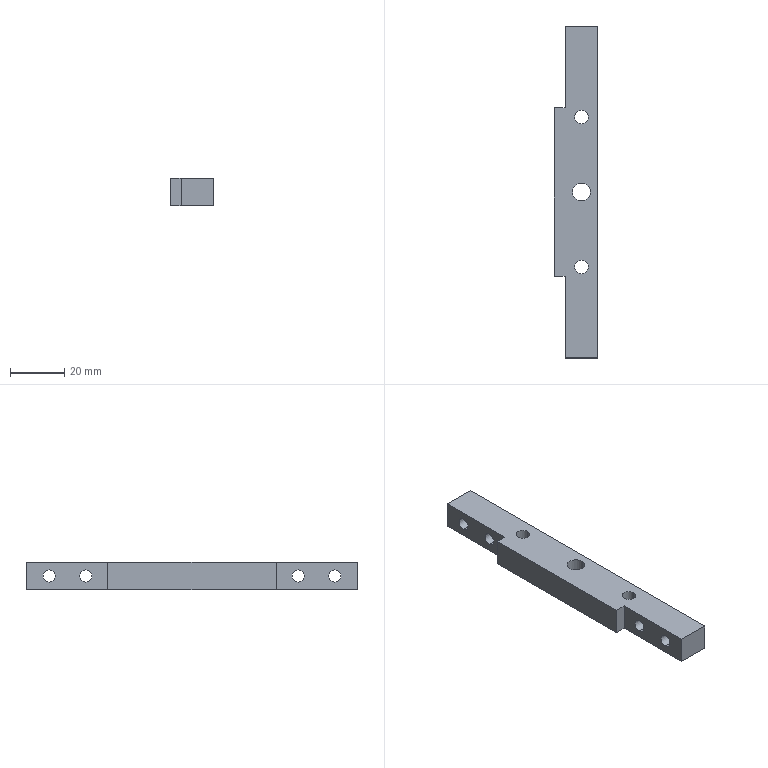Part | NX | features BREP 1 | 1 solid | 36 faces | box 16 x 122 x 10 mm | volume 15082 mm3 | cylinder 22 | plane 14 | commonest cylinder face diameters 4.5 x8 8 x8 5 x4 6.5 x2
STEP:
#1=CARTESIAN_POINT('',(-3.25,0.,0.));
#2=VERTEX_POINT('',#1);
#3=CARTESIAN_POINT('',(3.25,0.,0.));
#4=VERTEX_POINT('',#3);
#5=CARTESIAN_POINT('',(0.,0.,0.));
#6=DIRECTION('',(0.,0.,1.));
#7=DIRECTION('',(1.,0.,0.));
#8=AXIS2_PLACEMENT_3D('',#5,#6,#7);
#9=CIRCLE('',#8,3.25);
#10=EDGE_CURVE('',#2,#4,#9,.T.);
#11=ORIENTED_EDGE('',*,*,#10,.F.);
#12=CARTESIAN_POINT('',(-3.25,0.,10.));
#13=VERTEX_POINT('',#12);
#14=CARTESIAN_POINT('',(-3.25,0.,0.));
#15=DIRECTION('',(0.,0.,1.));
#16=VECTOR('',#15,1000.);
#17=LINE('',#14,#16);
#18=EDGE_CURVE('',#13,#2,#17,.F.);
#19=ORIENTED_EDGE('',*,*,#18,.F.);
#20=CARTESIAN_POINT('',(3.25,0.,10.));
#21=VERTEX_POINT('',#20);
#22=CARTESIAN_POINT('',(0.,0.,10.));
#23=DIRECTION('',(0.,0.,1.));
#24=DIRECTION('',(1.,0.,0.));
#25=AXIS2_PLACEMENT_3D('',#22,#23,#24);
#26=CIRCLE('',#25,3.25);
#27=EDGE_CURVE('',#13,#21,#26,.T.);
#28=ORIENTED_EDGE('',*,*,#27,.T.);
#29=CARTESIAN_POINT('',(3.25,0.,0.));
#30=DIRECTION('',(0.,0.,1.));
#31=VECTOR('',#30,1000.);
#32=LINE('',#29,#31);
#33=EDGE_CURVE('',#21,#4,#32,.F.);
#34=ORIENTED_EDGE('',*,*,#33,.T.);
#35=EDGE_LOOP('',(#11,#19,#28,#34));
#36=FACE_BOUND('',#35,.T.);
#37=CARTESIAN_POINT('',(0.,0.,0.));
#38=DIRECTION('',(0.,0.,1.));
#39=DIRECTION('',(1.,0.,0.));
#40=AXIS2_PLACEMENT_3D('',#37,#38,#39);
#41=CYLINDRICAL_SURFACE('',#40,3.25);
#42=ADVANCED_FACE('',(#36),#41,.F.);
#43=CARTESIAN_POINT('',(-2.5,27.5,0.));
#44=VERTEX_POINT('',#43);
#45=CARTESIAN_POINT('',(2.5,27.5,0.));
#46=VERTEX_POINT('',#45);
#47=CARTESIAN_POINT('',(0.,27.5,0.));
#48=DIRECTION('',(0.,0.,1.));
#49=DIRECTION('',(1.,0.,0.));
#50=AXIS2_PLACEMENT_3D('',#47,#48,#49);
#51=CIRCLE('',#50,2.5);
#52=EDGE_CURVE('',#44,#46,#51,.T.);
#53=ORIENTED_EDGE('',*,*,#52,.F.);
#54=CARTESIAN_POINT('',(-2.5,27.5,10.));
#55=VERTEX_POINT('',#54);
#56=CARTESIAN_POINT('',(-2.5,27.5,10.));
#57=DIRECTION('',(0.,0.,1.));
#58=VECTOR('',#57,1000.);
#59=LINE('',#56,#58);
#60=EDGE_CURVE('',#55,#44,#59,.F.);
#61=ORIENTED_EDGE('',*,*,#60,.F.);
#62=CARTESIAN_POINT('',(2.5,27.5,10.));
#63=VERTEX_POINT('',#62);
#64=CARTESIAN_POINT('',(0.,27.5,10.));
#65=DIRECTION('',(0.,0.,1.));
#66=DIRECTION('',(1.,0.,0.));
#67=AXIS2_PLACEMENT_3D('',#64,#65,#66);
#68=CIRCLE('',#67,2.5);
#69=EDGE_CURVE('',#55,#63,#68,.T.);
#70=ORIENTED_EDGE('',*,*,#69,.T.);
#71=CARTESIAN_POINT('',(2.5,27.5,10.));
#72=DIRECTION('',(0.,0.,1.));
#73=VECTOR('',#72,1000.);
#74=LINE('',#71,#73);
#75=EDGE_CURVE('',#63,#46,#74,.F.);
#76=ORIENTED_EDGE('',*,*,#75,.T.);
#77=EDGE_LOOP('',(#53,#61,#70,#76));
#78=FACE_BOUND('',#77,.T.);
#79=CARTESIAN_POINT('',(0.,27.5,10.));
#80=DIRECTION('',(0.,0.,1.));
#81=DIRECTION('',(1.,0.,0.));
#82=AXIS2_PLACEMENT_3D('',#79,#80,#81);
#83=CYLINDRICAL_SURFACE('',#82,2.5);
#84=ADVANCED_FACE('',(#78),#83,.F.);
#85=CARTESIAN_POINT('',(-2.5,-27.5,0.));
#86=VERTEX_POINT('',#85);
#87=CARTESIAN_POINT('',(2.5,-27.5,0.));
#88=VERTEX_POINT('',#87);
#89=CARTESIAN_POINT('',(0.,-27.5,0.));
#90=DIRECTION('',(0.,0.,1.));
#91=DIRECTION('',(1.,0.,0.));
#92=AXIS2_PLACEMENT_3D('',#89,#90,#91);
#93=CIRCLE('',#92,2.5);
#94=EDGE_CURVE('',#86,#88,#93,.T.);
#95=ORIENTED_EDGE('',*,*,#94,.F.);
#96=CARTESIAN_POINT('',(-2.5,-27.5,10.));
#97=VERTEX_POINT('',#96);
#98=CARTESIAN_POINT('',(-2.5,-27.5,10.));
#99=DIRECTION('',(0.,0.,1.));
#100=VECTOR('',#99,1000.);
#101=LINE('',#98,#100);
#102=EDGE_CURVE('',#97,#86,#101,.F.);
#103=ORIENTED_EDGE('',*,*,#102,.F.);
#104=CARTESIAN_POINT('',(2.5,-27.5,10.));
#105=VERTEX_POINT('',#104);
#106=CARTESIAN_POINT('',(0.,-27.5,10.));
#107=DIRECTION('',(0.,0.,1.));
#108=DIRECTION('',(1.,0.,0.));
#109=AXIS2_PLACEMENT_3D('',#106,#107,#108);
#110=CIRCLE('',#109,2.5);
#111=EDGE_CURVE('',#97,#105,#110,.T.);
#112=ORIENTED_EDGE('',*,*,#111,.T.);
#113=CARTESIAN_POINT('',(2.5,-27.5,10.));
#114=DIRECTION('',(0.,0.,1.));
#115=VECTOR('',#114,1000.);
#116=LINE('',#113,#115);
#117=EDGE_CURVE('',#105,#88,#116,.F.);
#118=ORIENTED_EDGE('',*,*,#117,.T.);
#119=EDGE_LOOP('',(#95,#103,#112,#118));
#120=FACE_BOUND('',#119,.T.);
#121=CARTESIAN_POINT('',(0.,-27.5,10.));
#122=DIRECTION('',(0.,0.,1.));
#123=DIRECTION('',(1.,0.,0.));
#124=AXIS2_PLACEMENT_3D('',#121,#122,#123);
#125=CYLINDRICAL_SURFACE('',#124,2.5);
#126=ADVANCED_FACE('',(#120),#125,.F.);
#127=CARTESIAN_POINT('',(2.,52.5,9.));
#128=VERTEX_POINT('',#127);
#129=CARTESIAN_POINT('',(2.,52.5,1.));
#130=VERTEX_POINT('',#129);
#131=CARTESIAN_POINT('',(2.,52.5,5.));
#132=DIRECTION('',(1.,0.,0.));
#133=DIRECTION('',(0.,0.,-1.));
#134=AXIS2_PLACEMENT_3D('',#131,#132,#133);
#135=CIRCLE('',#134,4.);
#136=EDGE_CURVE('',#128,#130,#135,.T.);
#137=ORIENTED_EDGE('',*,*,#136,.F.);
#138=CARTESIAN_POINT('',(6.,52.5,9.));
#139=VERTEX_POINT('',#138);
#140=CARTESIAN_POINT('',(6.,52.5,9.));
#141=DIRECTION('',(1.,0.,0.));
#142=VECTOR('',#141,1000.);
#143=LINE('',#140,#142);
#144=EDGE_CURVE('',#128,#139,#143,.T.);
#145=ORIENTED_EDGE('',*,*,#144,.T.);
#146=CARTESIAN_POINT('',(6.,52.5,1.));
#147=VERTEX_POINT('',#146);
#148=CARTESIAN_POINT('',(6.,52.5,5.));
#149=DIRECTION('',(1.,0.,0.));
#150=DIRECTION('',(0.,0.,-1.));
#151=AXIS2_PLACEMENT_3D('',#148,#149,#150);
#152=CIRCLE('',#151,4.);
#153=EDGE_CURVE('',#139,#147,#152,.T.);
#154=ORIENTED_EDGE('',*,*,#153,.T.);
#155=CARTESIAN_POINT('',(6.,52.5,1.));
#156=DIRECTION('',(1.,0.,0.));
#157=VECTOR('',#156,1000.);
#158=LINE('',#155,#157);
#159=EDGE_CURVE('',#130,#147,#158,.T.);
#160=ORIENTED_EDGE('',*,*,#159,.F.);
#161=EDGE_LOOP('',(#137,#145,#154,#160));
#162=FACE_BOUND('',#161,.T.);
#163=CARTESIAN_POINT('',(6.,52.5,5.));
#164=DIRECTION('',(1.,0.,0.));
#165=DIRECTION('',(0.,0.,-1.));
#166=AXIS2_PLACEMENT_3D('',#163,#164,#165);
#167=CYLINDRICAL_SURFACE('',#166,4.);
#168=ADVANCED_FACE('',(#162),#167,.F.);
#169=CARTESIAN_POINT('',(-6.,52.5,7.25));
#170=VERTEX_POINT('',#169);
#171=CARTESIAN_POINT('',(-6.,52.5,2.75));
#172=VERTEX_POINT('',#171);
#173=CARTESIAN_POINT('',(-6.,52.5,5.));
#174=DIRECTION('',(1.,0.,0.));
#175=DIRECTION('',(0.,1.,0.));
#176=AXIS2_PLACEMENT_3D('',#173,#174,#175);
#177=CIRCLE('',#176,2.25);
#178=EDGE_CURVE('',#170,#172,#177,.T.);
#179=ORIENTED_EDGE('',*,*,#178,.F.);
#180=CARTESIAN_POINT('',(2.,52.5,7.25));
#181=VERTEX_POINT('',#180);
#182=CARTESIAN_POINT('',(6.,52.5,7.25));
#183=DIRECTION('',(1.,0.,0.));
#184=VECTOR('',#183,1000.);
#185=LINE('',#182,#184);
#186=EDGE_CURVE('',#170,#181,#185,.T.);
#187=ORIENTED_EDGE('',*,*,#186,.T.);
#188=CARTESIAN_POINT('',(2.,52.5,2.75));
#189=VERTEX_POINT('',#188);
#190=CARTESIAN_POINT('',(2.,52.5,5.));
#191=DIRECTION('',(1.,0.,0.));
#192=DIRECTION('',(0.,0.,-1.));
#193=AXIS2_PLACEMENT_3D('',#190,#191,#192);
#194=CIRCLE('',#193,2.25);
#195=EDGE_CURVE('',#181,#189,#194,.T.);
#196=ORIENTED_EDGE('',*,*,#195,.T.);
#197=CARTESIAN_POINT('',(6.,52.5,2.75));
#198=DIRECTION('',(1.,0.,0.));
#199=VECTOR('',#198,1000.);
#200=LINE('',#197,#199);
#201=EDGE_CURVE('',#172,#189,#200,.T.);
#202=ORIENTED_EDGE('',*,*,#201,.F.);
#203=EDGE_LOOP('',(#179,#187,#196,#202));
#204=FACE_BOUND('',#203,.T.);
#205=CARTESIAN_POINT('',(6.,52.5,5.));
#206=DIRECTION('',(1.,0.,0.));
#207=DIRECTION('',(0.,0.,-1.));
#208=AXIS2_PLACEMENT_3D('',#205,#206,#207);
#209=CYLINDRICAL_SURFACE('',#208,2.25);
#210=ADVANCED_FACE('',(#204),#209,.F.);
#211=CARTESIAN_POINT('',(2.,39.,9.));
#212=VERTEX_POINT('',#211);
#213=CARTESIAN_POINT('',(2.,39.,1.));
#214=VERTEX_POINT('',#213);
#215=CARTESIAN_POINT('',(2.,39.,5.));
#216=DIRECTION('',(1.,0.,0.));
#217=DIRECTION('',(0.,0.,-1.));
#218=AXIS2_PLACEMENT_3D('',#215,#216,#217);
#219=CIRCLE('',#218,4.);
#220=EDGE_CURVE('',#212,#214,#219,.T.);
#221=ORIENTED_EDGE('',*,*,#220,.F.);
#222=CARTESIAN_POINT('',(6.,39.,9.));
#223=VERTEX_POINT('',#222);
#224=CARTESIAN_POINT('',(6.,39.,9.));
#225=DIRECTION('',(1.,0.,0.));
#226=VECTOR('',#225,1000.);
#227=LINE('',#224,#226);
#228=EDGE_CURVE('',#212,#223,#227,.T.);
#229=ORIENTED_EDGE('',*,*,#228,.T.);
#230=CARTESIAN_POINT('',(6.,39.,1.));
#231=VERTEX_POINT('',#230);
#232=CARTESIAN_POINT('',(6.,39.,5.));
#233=DIRECTION('',(1.,0.,0.));
#234=DIRECTION('',(0.,0.,-1.));
#235=AXIS2_PLACEMENT_3D('',#232,#233,#234);
#236=CIRCLE('',#235,4.);
#237=EDGE_CURVE('',#223,#231,#236,.T.);
#238=ORIENTED_EDGE('',*,*,#237,.T.);
#239=CARTESIAN_POINT('',(6.,39.,1.));
#240=DIRECTION('',(1.,0.,0.));
#241=VECTOR('',#240,1000.);
#242=LINE('',#239,#241);
#243=EDGE_CURVE('',#214,#231,#242,.T.);
#244=ORIENTED_EDGE('',*,*,#243,.F.);
#245=EDGE_LOOP('',(#221,#229,#238,#244));
#246=FACE_BOUND('',#245,.T.);
#247=CARTESIAN_POINT('',(6.,39.,5.));
#248=DIRECTION('',(1.,0.,0.));
#249=DIRECTION('',(0.,0.,-1.));
#250=AXIS2_PLACEMENT_3D('',#247,#248,#249);
#251=CYLINDRICAL_SURFACE('',#250,4.);
#252=ADVANCED_FACE('',(#246),#251,.F.);
#253=CARTESIAN_POINT('',(-6.,39.,7.25));
#254=VERTEX_POINT('',#253);
#255=CARTESIAN_POINT('',(-6.,39.,2.75));
#256=VERTEX_POINT('',#255);
#257=CARTESIAN_POINT('',(-6.,39.,5.));
#258=DIRECTION('',(1.,0.,0.));
#259=DIRECTION('',(0.,1.,0.));
#260=AXIS2_PLACEMENT_3D('',#257,#258,#259);
#261=CIRCLE('',#260,2.25);
#262=EDGE_CURVE('',#254,#256,#261,.T.);
#263=ORIENTED_EDGE('',*,*,#262,.F.);
#264=CARTESIAN_POINT('',(2.,39.,7.25));
#265=VERTEX_POINT('',#264);
#266=CARTESIAN_POINT('',(6.,39.,7.25));
#267=DIRECTION('',(1.,0.,0.));
#268=VECTOR('',#267,1000.);
#269=LINE('',#266,#268);
#270=EDGE_CURVE('',#254,#265,#269,.T.);
#271=ORIENTED_EDGE('',*,*,#270,.T.);
#272=CARTESIAN_POINT('',(2.,39.,2.75));
#273=VERTEX_POINT('',#272);
#274=CARTESIAN_POINT('',(2.,39.,5.));
#275=DIRECTION('',(1.,0.,0.));
#276=DIRECTION('',(0.,0.,-1.));
#277=AXIS2_PLACEMENT_3D('',#274,#275,#276);
#278=CIRCLE('',#277,2.25);
#279=EDGE_CURVE('',#265,#273,#278,.T.);
#280=ORIENTED_EDGE('',*,*,#279,.T.);
#281=CARTESIAN_POINT('',(6.,39.,2.75));
#282=DIRECTION('',(1.,0.,0.));
#283=VECTOR('',#282,1000.);
#284=LINE('',#281,#283);
#285=EDGE_CURVE('',#256,#273,#284,.T.);
#286=ORIENTED_EDGE('',*,*,#285,.F.);
#287=EDGE_LOOP('',(#263,#271,#280,#286));
#288=FACE_BOUND('',#287,.T.);
#289=CARTESIAN_POINT('',(6.,39.,5.));
#290=DIRECTION('',(1.,0.,0.));
#291=DIRECTION('',(0.,0.,-1.));
#292=AXIS2_PLACEMENT_3D('',#289,#290,#291);
#293=CYLINDRICAL_SURFACE('',#292,2.25);
#294=ADVANCED_FACE('',(#288),#293,.F.);
#295=CARTESIAN_POINT('',(2.,-39.,9.));
#296=VERTEX_POINT('',#295);
#297=CARTESIAN_POINT('',(2.,-39.,1.));
#298=VERTEX_POINT('',#297);
#299=CARTESIAN_POINT('',(2.,-39.,5.));
#300=DIRECTION('',(1.,0.,0.));
#301=DIRECTION('',(0.,0.,-1.));
#302=AXIS2_PLACEMENT_3D('',#299,#300,#301);
#303=CIRCLE('',#302,4.);
#304=EDGE_CURVE('',#296,#298,#303,.T.);
#305=ORIENTED_EDGE('',*,*,#304,.F.);
#306=CARTESIAN_POINT('',(6.,-39.,9.));
#307=VERTEX_POINT('',#306);
#308=CARTESIAN_POINT('',(6.,-39.,9.));
#309=DIRECTION('',(1.,0.,0.));
#310=VECTOR('',#309,1000.);
#311=LINE('',#308,#310);
#312=EDGE_CURVE('',#296,#307,#311,.T.);
#313=ORIENTED_EDGE('',*,*,#312,.T.);
#314=CARTESIAN_POINT('',(6.,-39.,1.));
#315=VERTEX_POINT('',#314);
#316=CARTESIAN_POINT('',(6.,-39.,5.));
#317=DIRECTION('',(1.,0.,0.));
#318=DIRECTION('',(0.,0.,-1.));
#319=AXIS2_PLACEMENT_3D('',#316,#317,#318);
#320=CIRCLE('',#319,4.);
#321=EDGE_CURVE('',#307,#315,#320,.T.);
#322=ORIENTED_EDGE('',*,*,#321,.T.);
#323=CARTESIAN_POINT('',(6.,-39.,1.));
#324=DIRECTION('',(1.,0.,0.));
#325=VECTOR('',#324,1000.);
#326=LINE('',#323,#325);
#327=EDGE_CURVE('',#298,#315,#326,.T.);
#328=ORIENTED_EDGE('',*,*,#327,.F.);
#329=EDGE_LOOP('',(#305,#313,#322,#328));
#330=FACE_BOUND('',#329,.T.);
#331=CARTESIAN_POINT('',(6.,-39.,5.));
#332=DIRECTION('',(1.,0.,0.));
#333=DIRECTION('',(0.,0.,-1.));
#334=AXIS2_PLACEMENT_3D('',#331,#332,#333);
#335=CYLINDRICAL_SURFACE('',#334,4.);
#336=ADVANCED_FACE('',(#330),#335,.F.);
#337=CARTESIAN_POINT('',(-6.,-39.,7.25));
#338=VERTEX_POINT('',#337);
#339=CARTESIAN_POINT('',(-6.,-39.,2.75));
#340=VERTEX_POINT('',#339);
#341=CARTESIAN_POINT('',(-6.,-39.,5.));
#342=DIRECTION('',(1.,0.,0.));
#343=DIRECTION('',(0.,1.,0.));
#344=AXIS2_PLACEMENT_3D('',#341,#342,#343);
#345=CIRCLE('',#344,2.25);
#346=EDGE_CURVE('',#338,#340,#345,.T.);
#347=ORIENTED_EDGE('',*,*,#346,.F.);
#348=CARTESIAN_POINT('',(2.,-39.,7.25));
#349=VERTEX_POINT('',#348);
#350=CARTESIAN_POINT('',(6.,-39.,7.25));
#351=DIRECTION('',(1.,0.,0.));
#352=VECTOR('',#351,1000.);
#353=LINE('',#350,#352);
#354=EDGE_CURVE('',#338,#349,#353,.T.);
#355=ORIENTED_EDGE('',*,*,#354,.T.);
#356=CARTESIAN_POINT('',(2.,-39.,2.75));
#357=VERTEX_POINT('',#356);
#358=CARTESIAN_POINT('',(2.,-39.,5.));
#359=DIRECTION('',(1.,0.,0.));
#360=DIRECTION('',(0.,0.,-1.));
#361=AXIS2_PLACEMENT_3D('',#358,#359,#360);
#362=CIRCLE('',#361,2.25);
#363=EDGE_CURVE('',#349,#357,#362,.T.);
#364=ORIENTED_EDGE('',*,*,#363,.T.);
#365=CARTESIAN_POINT('',(6.,-39.,2.75));
#366=DIRECTION('',(1.,0.,0.));
#367=VECTOR('',#366,1000.);
#368=LINE('',#365,#367);
#369=EDGE_CURVE('',#340,#357,#368,.T.);
#370=ORIENTED_EDGE('',*,*,#369,.F.);
#371=EDGE_LOOP('',(#347,#355,#364,#370));
#372=FACE_BOUND('',#371,.T.);
#373=CARTESIAN_POINT('',(6.,-39.,5.));
#374=DIRECTION('',(1.,0.,0.));
#375=DIRECTION('',(0.,0.,-1.));
#376=AXIS2_PLACEMENT_3D('',#373,#374,#375);
#377=CYLINDRICAL_SURFACE('',#376,2.25);
#378=ADVANCED_FACE('',(#372),#377,.F.);
#379=CARTESIAN_POINT('',(2.,-52.5,9.));
#380=VERTEX_POINT('',#379);
#381=CARTESIAN_POINT('',(2.,-52.5,1.));
#382=VERTEX_POINT('',#381);
#383=CARTESIAN_POINT('',(2.,-52.5,5.));
#384=DIRECTION('',(1.,0.,0.));
#385=DIRECTION('',(0.,0.,-1.));
#386=AXIS2_PLACEMENT_3D('',#383,#384,#385);
#387=CIRCLE('',#386,4.);
#388=EDGE_CURVE('',#380,#382,#387,.T.);
#389=ORIENTED_EDGE('',*,*,#388,.F.);
#390=CARTESIAN_POINT('',(6.,-52.5,9.));
#391=VERTEX_POINT('',#390);
#392=CARTESIAN_POINT('',(6.,-52.5,9.));
#393=DIRECTION('',(1.,0.,0.));
#394=VECTOR('',#393,1000.);
#395=LINE('',#392,#394);
#396=EDGE_CURVE('',#380,#391,#395,.T.);
#397=ORIENTED_EDGE('',*,*,#396,.T.);
#398=CARTESIAN_POINT('',(6.,-52.5,1.));
#399=VERTEX_POINT('',#398);
#400=CARTESIAN_POINT('',(6.,-52.5,5.));
#401=DIRECTION('',(1.,0.,0.));
#402=DIRECTION('',(0.,0.,-1.));
#403=AXIS2_PLACEMENT_3D('',#400,#401,#402);
#404=CIRCLE('',#403,4.);
#405=EDGE_CURVE('',#391,#399,#404,.T.);
#406=ORIENTED_EDGE('',*,*,#405,.T.);
#407=CARTESIAN_POINT('',(6.,-52.5,1.));
#408=DIRECTION('',(1.,0.,0.));
#409=VECTOR('',#408,1000.);
#410=LINE('',#407,#409);
#411=EDGE_CURVE('',#382,#399,#410,.T.);
#412=ORIENTED_EDGE('',*,*,#411,.F.);
#413=EDGE_LOOP('',(#389,#397,#406,#412));
#414=FACE_BOUND('',#413,.T.);
#415=CARTESIAN_POINT('',(6.,-52.5,5.));
#416=DIRECTION('',(1.,0.,0.));
#417=DIRECTION('',(0.,0.,-1.));
#418=AXIS2_PLACEMENT_3D('',#415,#416,#417);
#419=CYLINDRICAL_SURFACE('',#418,4.);
#420=ADVANCED_FACE('',(#414),#419,.F.);
#421=CARTESIAN_POINT('',(-6.,-52.5,7.25));
#422=VERTEX_POINT('',#421);
#423=CARTESIAN_POINT('',(-6.,-52.5,2.75));
#424=VERTEX_POINT('',#423);
#425=CARTESIAN_POINT('',(-6.,-52.5,5.));
#426=DIRECTION('',(1.,0.,0.));
#427=DIRECTION('',(0.,1.,0.));
#428=AXIS2_PLACEMENT_3D('',#425,#426,#427);
#429=CIRCLE('',#428,2.25);
#430=EDGE_CURVE('',#422,#424,#429,.T.);
#431=ORIENTED_EDGE('',*,*,#430,.F.);
#432=CARTESIAN_POINT('',(2.,-52.5,7.25));
#433=VERTEX_POINT('',#432);
#434=CARTESIAN_POINT('',(6.,-52.5,7.25));
#435=DIRECTION('',(1.,0.,0.));
#436=VECTOR('',#435,1000.);
#437=LINE('',#434,#436);
#438=EDGE_CURVE('',#422,#433,#437,.T.);
#439=ORIENTED_EDGE('',*,*,#438,.T.);
#440=CARTESIAN_POINT('',(2.,-52.5,2.75));
#441=VERTEX_POINT('',#440);
#442=CARTESIAN_POINT('',(2.,-52.5,5.));
#443=DIRECTION('',(1.,0.,0.));
#444=DIRECTION('',(0.,0.,-1.));
#445=AXIS2_PLACEMENT_3D('',#442,#443,#444);
#446=CIRCLE('',#445,2.25);
#447=EDGE_CURVE('',#433,#441,#446,.T.);
#448=ORIENTED_EDGE('',*,*,#447,.T.);
#449=CARTESIAN_POINT('',(6.,-52.5,2.75));
#450=DIRECTION('',(1.,0.,0.));
#451=VECTOR('',#450,1000.);
#452=LINE('',#449,#451);
#453=EDGE_CURVE('',#424,#441,#452,.T.);
#454=ORIENTED_EDGE('',*,*,#453,.F.);
#455=EDGE_LOOP('',(#431,#439,#448,#454));
#456=FACE_BOUND('',#455,.T.);
#457=CARTESIAN_POINT('',(6.,-52.5,5.));
#458=DIRECTION('',(1.,0.,0.));
#459=DIRECTION('',(0.,0.,-1.));
#460=AXIS2_PLACEMENT_3D('',#457,#458,#459);
#461=CYLINDRICAL_SURFACE('',#460,2.25);
#462=ADVANCED_FACE('',(#456),#461,.F.);
#463=CARTESIAN_POINT('',(6.,-61.,0.));
#464=VERTEX_POINT('',#463);
#465=CARTESIAN_POINT('',(6.,61.,0.));
#466=VERTEX_POINT('',#465);
#467=CARTESIAN_POINT('',(6.,61.,0.));
#468=DIRECTION('',(0.,1.,0.));
#469=VECTOR('',#468,1000.);
#470=LINE('',#467,#469);
#471=EDGE_CURVE('',#464,#466,#470,.T.);
#472=ORIENTED_EDGE('',*,*,#471,.T.);
#473=CARTESIAN_POINT('',(6.,61.,10.));
#474=VERTEX_POINT('',#473);
#475=CARTESIAN_POINT('',(6.,61.,10.));
#476=DIRECTION('',(0.,0.,-1.));
#477=VECTOR('',#476,1000.);
#478=LINE('',#475,#477);
#479=EDGE_CURVE('',#474,#466,#478,.T.);
#480=ORIENTED_EDGE('',*,*,#479,.F.);
#481=CARTESIAN_POINT('',(6.,-61.,10.));
#482=VERTEX_POINT('',#481);
#483=CARTESIAN_POINT('',(6.,61.,10.));
#484=DIRECTION('',(0.,1.,0.));
#485=VECTOR('',#484,1000.);
#486=LINE('',#483,#485);
#487=EDGE_CURVE('',#482,#474,#486,.T.);
#488=ORIENTED_EDGE('',*,*,#487,.F.);
#489=CARTESIAN_POINT('',(6.,-61.,10.));
#490=DIRECTION('',(0.,0.,-1.));
#491=VECTOR('',#490,1000.);
#492=LINE('',#489,#491);
#493=EDGE_CURVE('',#482,#464,#492,.T.);
#494=ORIENTED_EDGE('',*,*,#493,.T.);
#495=EDGE_LOOP('',(#472,#480,#488,#494));
#496=FACE_BOUND('',#495,.T.);
#497=CARTESIAN_POINT('',(6.,52.5,5.));
#498=DIRECTION('',(1.,0.,0.));
#499=DIRECTION('',(0.,0.,-1.));
#500=AXIS2_PLACEMENT_3D('',#497,#498,#499);
#501=CIRCLE('',#500,4.);
#502=EDGE_CURVE('',#147,#139,#501,.T.);
#503=ORIENTED_EDGE('',*,*,#502,.F.);
#504=ORIENTED_EDGE('',*,*,#153,.F.);
#505=EDGE_LOOP('',(#503,#504));
#506=FACE_BOUND('',#505,.T.);
#507=CARTESIAN_POINT('',(6.,39.,5.));
#508=DIRECTION('',(1.,0.,0.));
#509=DIRECTION('',(0.,0.,-1.));
#510=AXIS2_PLACEMENT_3D('',#507,#508,#509);
#511=CIRCLE('',#510,4.);
#512=EDGE_CURVE('',#231,#223,#511,.T.);
#513=ORIENTED_EDGE('',*,*,#512,.F.);
#514=ORIENTED_EDGE('',*,*,#237,.F.);
#515=EDGE_LOOP('',(#513,#514));
#516=FACE_BOUND('',#515,.T.);
#517=CARTESIAN_POINT('',(6.,-39.,5.));
#518=DIRECTION('',(1.,0.,0.));
#519=DIRECTION('',(0.,0.,-1.));
#520=AXIS2_PLACEMENT_3D('',#517,#518,#519);
#521=CIRCLE('',#520,4.);
#522=EDGE_CURVE('',#315,#307,#521,.T.);
#523=ORIENTED_EDGE('',*,*,#522,.F.);
#524=ORIENTED_EDGE('',*,*,#321,.F.);
#525=EDGE_LOOP('',(#523,#524));
#526=FACE_BOUND('',#525,.T.);
#527=CARTESIAN_POINT('',(6.,-52.5,5.));
#528=DIRECTION('',(1.,0.,0.));
#529=DIRECTION('',(0.,0.,-1.));
#530=AXIS2_PLACEMENT_3D('',#527,#528,#529);
#531=CIRCLE('',#530,4.);
#532=EDGE_CURVE('',#399,#391,#531,.T.);
#533=ORIENTED_EDGE('',*,*,#532,.F.);
#534=ORIENTED_EDGE('',*,*,#405,.F.);
#535=EDGE_LOOP('',(#533,#534));
#536=FACE_BOUND('',#535,.T.);
#537=CARTESIAN_POINT('',(6.,61.,10.));
#538=DIRECTION('',(-1.,0.,0.));
#539=DIRECTION('',(0.,0.,1.));
#540=AXIS2_PLACEMENT_3D('',#537,#538,#539);
#541=PLANE('',#540);
#542=ADVANCED_FACE('',(#496,#506,#516,#526,#536),#541,.F.);
#543=CARTESIAN_POINT('',(-6.,61.,0.));
#544=VERTEX_POINT('',#543);
#545=CARTESIAN_POINT('',(6.,61.,0.));
#546=DIRECTION('',(-1.,0.,0.));
#547=VECTOR('',#546,1000.);
#548=LINE('',#545,#547);
#549=EDGE_CURVE('',#466,#544,#548,.T.);
#550=ORIENTED_EDGE('',*,*,#549,.T.);
#551=CARTESIAN_POINT('',(-6.,61.,10.));
#552=VERTEX_POINT('',#551);
#553=CARTESIAN_POINT('',(-6.,61.,10.));
#554=DIRECTION('',(0.,0.,-1.));
#555=VECTOR('',#554,1000.);
#556=LINE('',#553,#555);
#557=EDGE_CURVE('',#552,#544,#556,.T.);
#558=ORIENTED_EDGE('',*,*,#557,.F.);
#559=CARTESIAN_POINT('',(6.,61.,10.));
#560=DIRECTION('',(-1.,0.,0.));
#561=VECTOR('',#560,1000.);
#562=LINE('',#559,#561);
#563=EDGE_CURVE('',#474,#552,#562,.T.);
#564=ORIENTED_EDGE('',*,*,#563,.F.);
#565=ORIENTED_EDGE('',*,*,#479,.T.);
#566=EDGE_LOOP('',(#550,#558,#564,#565));
#567=FACE_BOUND('',#566,.T.);
#568=CARTESIAN_POINT('',(6.,61.,10.));
#569=DIRECTION('',(0.,-1.,0.));
#570=DIRECTION('',(0.,0.,-1.));
#571=AXIS2_PLACEMENT_3D('',#568,#569,#570);
#572=PLANE('',#571);
#573=ADVANCED_FACE('',(#567),#572,.F.);
#574=CARTESIAN_POINT('',(-6.,31.,0.));
#575=VERTEX_POINT('',#574);
#576=CARTESIAN_POINT('',(-6.,61.,0.));
#577=DIRECTION('',(0.,-1.,0.));
#578=VECTOR('',#577,1000.);
#579=LINE('',#576,#578);
#580=EDGE_CURVE('',#544,#575,#579,.T.);
#581=ORIENTED_EDGE('',*,*,#580,.T.);
#582=CARTESIAN_POINT('',(-6.,31.,10.));
#583=VERTEX_POINT('',#582);
#584=CARTESIAN_POINT('',(-6.,31.,10.));
#585=DIRECTION('',(0.,0.,-1.));
#586=VECTOR('',#585,1000.);
#587=LINE('',#584,#586);
#588=EDGE_CURVE('',#583,#575,#587,.T.);
#589=ORIENTED_EDGE('',*,*,#588,.F.);
#590=CARTESIAN_POINT('',(-6.,61.,10.));
#591=DIRECTION('',(0.,-1.,0.));
#592=VECTOR('',#591,1000.);
#593=LINE('',#590,#592);
#594=EDGE_CURVE('',#552,#583,#593,.T.);
#595=ORIENTED_EDGE('',*,*,#594,.F.);
#596=ORIENTED_EDGE('',*,*,#557,.T.);
#597=EDGE_LOOP('',(#581,#589,#595,#596));
#598=FACE_BOUND('',#597,.T.);
#599=CARTESIAN_POINT('',(-6.,52.5,5.));
#600=DIRECTION('',(1.,0.,0.));
#601=DIRECTION('',(0.,1.,0.));
#602=AXIS2_PLACEMENT_3D('',#599,#600,#601);
#603=CIRCLE('',#602,2.25);
#604=EDGE_CURVE('',#172,#170,#603,.T.);
#605=ORIENTED_EDGE('',*,*,#604,.T.);
#606=ORIENTED_EDGE('',*,*,#178,.T.);
#607=EDGE_LOOP('',(#605,#606));
#608=FACE_BOUND('',#607,.T.);
#609=CARTESIAN_POINT('',(-6.,39.,5.));
#610=DIRECTION('',(1.,0.,0.));
#611=DIRECTION('',(0.,1.,0.));
#612=AXIS2_PLACEMENT_3D('',#609,#610,#611);
#613=CIRCLE('',#612,2.25);
#614=EDGE_CURVE('',#256,#254,#613,.T.);
#615=ORIENTED_EDGE('',*,*,#614,.T.);
#616=ORIENTED_EDGE('',*,*,#262,.T.);
#617=EDGE_LOOP('',(#615,#616));
#618=FACE_BOUND('',#617,.T.);
#619=CARTESIAN_POINT('',(-6.,61.,10.));
#620=DIRECTION('',(1.,0.,0.));
#621=DIRECTION('',(0.,1.,0.));
#622=AXIS2_PLACEMENT_3D('',#619,#620,#621);
#623=PLANE('',#622);
#624=ADVANCED_FACE('',(#598,#608,#618),#623,.F.);
#625=CARTESIAN_POINT('',(-10.,31.,0.));
#626=VERTEX_POINT('',#625);
#627=CARTESIAN_POINT('',(-6.,31.,0.));
#628=DIRECTION('',(-1.,0.,0.));
#629=VECTOR('',#628,1000.);
#630=LINE('',#627,#629);
#631=EDGE_CURVE('',#575,#626,#630,.T.);
#632=ORIENTED_EDGE('',*,*,#631,.T.);
#633=CARTESIAN_POINT('',(-10.,31.,10.));
#634=VERTEX_POINT('',#633);
#635=CARTESIAN_POINT('',(-10.,31.,10.));
#636=DIRECTION('',(0.,0.,-1.));
#637=VECTOR('',#636,1000.);
#638=LINE('',#635,#637);
#639=EDGE_CURVE('',#634,#626,#638,.T.);
#640=ORIENTED_EDGE('',*,*,#639,.F.);
#641=CARTESIAN_POINT('',(-6.,31.,10.));
#642=DIRECTION('',(-1.,0.,0.));
#643=VECTOR('',#642,1000.);
#644=LINE('',#641,#643);
#645=EDGE_CURVE('',#583,#634,#644,.T.);
#646=ORIENTED_EDGE('',*,*,#645,.F.);
#647=ORIENTED_EDGE('',*,*,#588,.T.);
#648=EDGE_LOOP('',(#632,#640,#646,#647));
#649=FACE_BOUND('',#648,.T.);
#650=CARTESIAN_POINT('',(-6.,31.,10.));
#651=DIRECTION('',(0.,-1.,0.));
#652=DIRECTION('',(0.,0.,-1.));
#653=AXIS2_PLACEMENT_3D('',#650,#651,#652);
#654=PLANE('',#653);
#655=ADVANCED_FACE('',(#649),#654,.F.);
#656=CARTESIAN_POINT('',(-10.,-31.,0.));
#657=VERTEX_POINT('',#656);
#658=CARTESIAN_POINT('',(-10.,31.,0.));
#659=DIRECTION('',(0.,-1.,0.));
#660=VECTOR('',#659,1000.);
#661=LINE('',#658,#660);
#662=EDGE_CURVE('',#626,#657,#661,.T.);
#663=ORIENTED_EDGE('',*,*,#662,.T.);
#664=CARTESIAN_POINT('',(-10.,-31.,10.));
#665=VERTEX_POINT('',#664);
#666=CARTESIAN_POINT('',(-10.,-31.,10.));
#667=DIRECTION('',(0.,0.,-1.));
#668=VECTOR('',#667,1000.);
#669=LINE('',#666,#668);
#670=EDGE_CURVE('',#665,#657,#669,.T.);
#671=ORIENTED_EDGE('',*,*,#670,.F.);
#672=CARTESIAN_POINT('',(-10.,31.,10.));
#673=DIRECTION('',(0.,-1.,0.));
#674=VECTOR('',#673,1000.);
#675=LINE('',#672,#674);
#676=EDGE_CURVE('',#634,#665,#675,.T.);
#677=ORIENTED_EDGE('',*,*,#676,.F.);
#678=ORIENTED_EDGE('',*,*,#639,.T.);
#679=EDGE_LOOP('',(#663,#671,#677,#678));
#680=FACE_BOUND('',#679,.T.);
#681=CARTESIAN_POINT('',(-10.,31.,10.));
#682=DIRECTION('',(1.,0.,0.));
#683=DIRECTION('',(0.,1.,0.));
#684=AXIS2_PLACEMENT_3D('',#681,#682,#683);
#685=PLANE('',#684);
#686=ADVANCED_FACE('',(#680),#685,.F.);
#687=CARTESIAN_POINT('',(-6.,-31.,0.));
#688=VERTEX_POINT('',#687);
#689=CARTESIAN_POINT('',(-6.,-31.,0.));
#690=DIRECTION('',(1.,0.,0.));
#691=VECTOR('',#690,1000.);
#692=LINE('',#689,#691);
#693=EDGE_CURVE('',#657,#688,#692,.T.);
#694=ORIENTED_EDGE('',*,*,#693,.T.);
#695=CARTESIAN_POINT('',(-6.,-31.,10.));
#696=VERTEX_POINT('',#695);
#697=CARTESIAN_POINT('',(-6.,-31.,10.));
#698=DIRECTION('',(0.,0.,-1.));
#699=VECTOR('',#698,1000.);
#700=LINE('',#697,#699);
#701=EDGE_CURVE('',#696,#688,#700,.T.);
#702=ORIENTED_EDGE('',*,*,#701,.F.);
#703=CARTESIAN_POINT('',(-6.,-31.,10.));
#704=DIRECTION('',(1.,0.,0.));
#705=VECTOR('',#704,1000.);
#706=LINE('',#703,#705);
#707=EDGE_CURVE('',#665,#696,#706,.T.);
#708=ORIENTED_EDGE('',*,*,#707,.F.);
#709=ORIENTED_EDGE('',*,*,#670,.T.);
#710=EDGE_LOOP('',(#694,#702,#708,#709));
#711=FACE_BOUND('',#710,.T.);
#712=CARTESIAN_POINT('',(-6.,-31.,10.));
#713=DIRECTION('',(0.,1.,0.));
#714=DIRECTION('',(1.,0.,0.));
#715=AXIS2_PLACEMENT_3D('',#712,#713,#714);
#716=PLANE('',#715);
#717=ADVANCED_FACE('',(#711),#716,.F.);
#718=CARTESIAN_POINT('',(-6.,-61.,0.));
#719=VERTEX_POINT('',#718);
#720=CARTESIAN_POINT('',(-6.,-31.,0.));
#721=DIRECTION('',(0.,-1.,0.));
#722=VECTOR('',#721,1000.);
#723=LINE('',#720,#722);
#724=EDGE_CURVE('',#688,#719,#723,.T.);
#725=ORIENTED_EDGE('',*,*,#724,.T.);
#726=CARTESIAN_POINT('',(-6.,-61.,10.));
#727=VERTEX_POINT('',#726);
#728=CARTESIAN_POINT('',(-6.,-61.,10.));
#729=DIRECTION('',(0.,0.,-1.));
#730=VECTOR('',#729,1000.);
#731=LINE('',#728,#730);
#732=EDGE_CURVE('',#727,#719,#731,.T.);
#733=ORIENTED_EDGE('',*,*,#732,.F.);
#734=CARTESIAN_POINT('',(-6.,-31.,10.));
#735=DIRECTION('',(0.,-1.,0.));
#736=VECTOR('',#735,1000.);
#737=LINE('',#734,#736);
#738=EDGE_CURVE('',#696,#727,#737,.T.);
#739=ORIENTED_EDGE('',*,*,#738,.F.);
#740=ORIENTED_EDGE('',*,*,#701,.T.);
#741=EDGE_LOOP('',(#725,#733,#739,#740));
#742=FACE_BOUND('',#741,.T.);
#743=CARTESIAN_POINT('',(-6.,-39.,5.));
#744=DIRECTION('',(1.,0.,0.));
#745=DIRECTION('',(0.,1.,0.));
#746=AXIS2_PLACEMENT_3D('',#743,#744,#745);
#747=CIRCLE('',#746,2.25);
#748=EDGE_CURVE('',#340,#338,#747,.T.);
#749=ORIENTED_EDGE('',*,*,#748,.T.);
#750=ORIENTED_EDGE('',*,*,#346,.T.);
#751=EDGE_LOOP('',(#749,#750));
#752=FACE_BOUND('',#751,.T.);
#753=CARTESIAN_POINT('',(-6.,-52.5,5.));
#754=DIRECTION('',(1.,0.,0.));
#755=DIRECTION('',(0.,1.,0.));
#756=AXIS2_PLACEMENT_3D('',#753,#754,#755);
#757=CIRCLE('',#756,2.25);
#758=EDGE_CURVE('',#424,#422,#757,.T.);
#759=ORIENTED_EDGE('',*,*,#758,.T.);
#760=ORIENTED_EDGE('',*,*,#430,.T.);
#761=EDGE_LOOP('',(#759,#760));
#762=FACE_BOUND('',#761,.T.);
#763=CARTESIAN_POINT('',(-6.,-31.,10.));
#764=DIRECTION('',(1.,0.,0.));
#765=DIRECTION('',(0.,-1.,0.));
#766=AXIS2_PLACEMENT_3D('',#763,#764,#765);
#767=PLANE('',#766);
#768=ADVANCED_FACE('',(#742,#752,#762),#767,.F.);
#769=CARTESIAN_POINT('',(6.,-61.,0.));
#770=DIRECTION('',(1.,0.,0.));
#771=VECTOR('',#770,1000.);
#772=LINE('',#769,#771);
#773=EDGE_CURVE('',#719,#464,#772,.T.);
#774=ORIENTED_EDGE('',*,*,#773,.T.);
#775=ORIENTED_EDGE('',*,*,#493,.F.);
#776=CARTESIAN_POINT('',(6.,-61.,10.));
#777=DIRECTION('',(1.,0.,0.));
#778=VECTOR('',#777,1000.);
#779=LINE('',#776,#778);
#780=EDGE_CURVE('',#727,#482,#779,.T.);
#781=ORIENTED_EDGE('',*,*,#780,.F.);
#782=ORIENTED_EDGE('',*,*,#732,.T.);
#783=EDGE_LOOP('',(#774,#775,#781,#782));
#784=FACE_BOUND('',#783,.T.);
#785=CARTESIAN_POINT('',(6.,-61.,10.));
#786=DIRECTION('',(0.,1.,0.));
#787=DIRECTION('',(1.,0.,0.));
#788=AXIS2_PLACEMENT_3D('',#785,#786,#787);
#789=PLANE('',#788);
#790=ADVANCED_FACE('',(#784),#789,.F.);
#791=ORIENTED_EDGE('',*,*,#487,.T.);
#792=ORIENTED_EDGE('',*,*,#563,.T.);
#793=ORIENTED_EDGE('',*,*,#594,.T.);
#794=ORIENTED_EDGE('',*,*,#645,.T.);
#795=ORIENTED_EDGE('',*,*,#676,.T.);
#796=ORIENTED_EDGE('',*,*,#707,.T.);
#797=ORIENTED_EDGE('',*,*,#738,.T.);
#798=ORIENTED_EDGE('',*,*,#780,.T.);
#799=EDGE_LOOP('',(#791,#792,#793,#794,#795,#796,#797,#798));
#800=FACE_BOUND('',#799,.T.);
#801=CARTESIAN_POINT('',(0.,0.,10.));
#802=DIRECTION('',(0.,0.,1.));
#803=DIRECTION('',(1.,0.,0.));
#804=AXIS2_PLACEMENT_3D('',#801,#802,#803);
#805=CIRCLE('',#804,3.25);
#806=EDGE_CURVE('',#21,#13,#805,.T.);
#807=ORIENTED_EDGE('',*,*,#806,.F.);
#808=ORIENTED_EDGE('',*,*,#27,.F.);
#809=EDGE_LOOP('',(#807,#808));
#810=FACE_BOUND('',#809,.T.);
#811=CARTESIAN_POINT('',(0.,27.5,10.));
#812=DIRECTION('',(0.,0.,1.));
#813=DIRECTION('',(1.,0.,0.));
#814=AXIS2_PLACEMENT_3D('',#811,#812,#813);
#815=CIRCLE('',#814,2.5);
#816=EDGE_CURVE('',#63,#55,#815,.T.);
#817=ORIENTED_EDGE('',*,*,#816,.F.);
#818=ORIENTED_EDGE('',*,*,#69,.F.);
#819=EDGE_LOOP('',(#817,#818));
#820=FACE_BOUND('',#819,.T.);
#821=CARTESIAN_POINT('',(0.,-27.5,10.));
#822=DIRECTION('',(0.,0.,1.));
#823=DIRECTION('',(1.,0.,0.));
#824=AXIS2_PLACEMENT_3D('',#821,#822,#823);
#825=CIRCLE('',#824,2.5);
#826=EDGE_CURVE('',#105,#97,#825,.T.);
#827=ORIENTED_EDGE('',*,*,#826,.F.);
#828=ORIENTED_EDGE('',*,*,#111,.F.);
#829=EDGE_LOOP('',(#827,#828));
#830=FACE_BOUND('',#829,.T.);
#831=CARTESIAN_POINT('',(6.,-61.,10.));
#832=DIRECTION('',(0.,0.,-1.));
#833=DIRECTION('',(0.,-1.,0.));
#834=AXIS2_PLACEMENT_3D('',#831,#832,#833);
#835=PLANE('',#834);
#836=ADVANCED_FACE('',(#800,#810,#820,#830),#835,.F.);
#837=ORIENTED_EDGE('',*,*,#471,.F.);
#838=ORIENTED_EDGE('',*,*,#773,.F.);
#839=ORIENTED_EDGE('',*,*,#724,.F.);
#840=ORIENTED_EDGE('',*,*,#693,.F.);
#841=ORIENTED_EDGE('',*,*,#662,.F.);
#842=ORIENTED_EDGE('',*,*,#631,.F.);
#843=ORIENTED_EDGE('',*,*,#580,.F.);
#844=ORIENTED_EDGE('',*,*,#549,.F.);
#845=EDGE_LOOP('',(#837,#838,#839,#840,#841,#842,#843,#844));
#846=FACE_BOUND('',#845,.T.);
#847=CARTESIAN_POINT('',(0.,0.,0.));
#848=DIRECTION('',(0.,0.,1.));
#849=DIRECTION('',(1.,0.,0.));
#850=AXIS2_PLACEMENT_3D('',#847,#848,#849);
#851=CIRCLE('',#850,3.25);
#852=EDGE_CURVE('',#4,#2,#851,.T.);
#853=ORIENTED_EDGE('',*,*,#852,.T.);
#854=ORIENTED_EDGE('',*,*,#10,.T.);
#855=EDGE_LOOP('',(#853,#854));
#856=FACE_BOUND('',#855,.T.);
#857=CARTESIAN_POINT('',(0.,27.5,0.));
#858=DIRECTION('',(0.,0.,1.));
#859=DIRECTION('',(1.,0.,0.));
#860=AXIS2_PLACEMENT_3D('',#857,#858,#859);
#861=CIRCLE('',#860,2.5);
#862=EDGE_CURVE('',#46,#44,#861,.T.);
#863=ORIENTED_EDGE('',*,*,#862,.T.);
#864=ORIENTED_EDGE('',*,*,#52,.T.);
#865=EDGE_LOOP('',(#863,#864));
#866=FACE_BOUND('',#865,.T.);
#867=CARTESIAN_POINT('',(0.,-27.5,0.));
#868=DIRECTION('',(0.,0.,1.));
#869=DIRECTION('',(1.,0.,0.));
#870=AXIS2_PLACEMENT_3D('',#867,#868,#869);
#871=CIRCLE('',#870,2.5);
#872=EDGE_CURVE('',#88,#86,#871,.T.);
#873=ORIENTED_EDGE('',*,*,#872,.T.);
#874=ORIENTED_EDGE('',*,*,#94,.T.);
#875=EDGE_LOOP('',(#873,#874));
#876=FACE_BOUND('',#875,.T.);
#877=CARTESIAN_POINT('',(6.,-61.,0.));
#878=DIRECTION('',(0.,0.,-1.));
#879=DIRECTION('',(0.,-1.,0.));
#880=AXIS2_PLACEMENT_3D('',#877,#878,#879);
#881=PLANE('',#880);
#882=ADVANCED_FACE('',(#846,#856,#866,#876),#881,.T.);
#883=ORIENTED_EDGE('',*,*,#438,.F.);
#884=ORIENTED_EDGE('',*,*,#758,.F.);
#885=ORIENTED_EDGE('',*,*,#453,.T.);
#886=CARTESIAN_POINT('',(2.,-52.5,5.));
#887=DIRECTION('',(1.,0.,0.));
#888=DIRECTION('',(0.,0.,-1.));
#889=AXIS2_PLACEMENT_3D('',#886,#887,#888);
#890=CIRCLE('',#889,2.25);
#891=EDGE_CURVE('',#441,#433,#890,.T.);
#892=ORIENTED_EDGE('',*,*,#891,.T.);
#893=EDGE_LOOP('',(#883,#884,#885,#892));
#894=FACE_BOUND('',#893,.T.);
#895=CARTESIAN_POINT('',(6.,-52.5,5.));
#896=DIRECTION('',(1.,0.,0.));
#897=DIRECTION('',(0.,0.,-1.));
#898=AXIS2_PLACEMENT_3D('',#895,#896,#897);
#899=CYLINDRICAL_SURFACE('',#898,2.25);
#900=ADVANCED_FACE('',(#894),#899,.F.);
#901=CARTESIAN_POINT('',(2.,-52.5,5.));
#902=DIRECTION('',(1.,0.,0.));
#903=DIRECTION('',(0.,0.,-1.));
#904=AXIS2_PLACEMENT_3D('',#901,#902,#903);
#905=CIRCLE('',#904,4.);
#906=EDGE_CURVE('',#382,#380,#905,.T.);
#907=ORIENTED_EDGE('',*,*,#906,.T.);
#908=ORIENTED_EDGE('',*,*,#388,.T.);
#909=EDGE_LOOP('',(#907,#908));
#910=FACE_BOUND('',#909,.T.);
#911=ORIENTED_EDGE('',*,*,#891,.F.);
#912=ORIENTED_EDGE('',*,*,#447,.F.);
#913=EDGE_LOOP('',(#911,#912));
#914=FACE_BOUND('',#913,.T.);
#915=CARTESIAN_POINT('',(2.,-50.25,5.));
#916=DIRECTION('',(-1.,0.,0.));
#917=DIRECTION('',(0.,0.,1.));
#918=AXIS2_PLACEMENT_3D('',#915,#916,#917);
#919=PLANE('',#918);
#920=ADVANCED_FACE('',(#910,#914),#919,.F.);
#921=ORIENTED_EDGE('',*,*,#396,.F.);
#922=ORIENTED_EDGE('',*,*,#906,.F.);
#923=ORIENTED_EDGE('',*,*,#411,.T.);
#924=ORIENTED_EDGE('',*,*,#532,.T.);
#925=EDGE_LOOP('',(#921,#922,#923,#924));
#926=FACE_BOUND('',#925,.T.);
#927=CARTESIAN_POINT('',(6.,-52.5,5.));
#928=DIRECTION('',(1.,0.,0.));
#929=DIRECTION('',(0.,0.,-1.));
#930=AXIS2_PLACEMENT_3D('',#927,#928,#929);
#931=CYLINDRICAL_SURFACE('',#930,4.);
#932=ADVANCED_FACE('',(#926),#931,.F.);
#933=ORIENTED_EDGE('',*,*,#354,.F.);
#934=ORIENTED_EDGE('',*,*,#748,.F.);
#935=ORIENTED_EDGE('',*,*,#369,.T.);
#936=CARTESIAN_POINT('',(2.,-39.,5.));
#937=DIRECTION('',(1.,0.,0.));
#938=DIRECTION('',(0.,0.,-1.));
#939=AXIS2_PLACEMENT_3D('',#936,#937,#938);
#940=CIRCLE('',#939,2.25);
#941=EDGE_CURVE('',#357,#349,#940,.T.);
#942=ORIENTED_EDGE('',*,*,#941,.T.);
#943=EDGE_LOOP('',(#933,#934,#935,#942));
#944=FACE_BOUND('',#943,.T.);
#945=CARTESIAN_POINT('',(6.,-39.,5.));
#946=DIRECTION('',(1.,0.,0.));
#947=DIRECTION('',(0.,0.,-1.));
#948=AXIS2_PLACEMENT_3D('',#945,#946,#947);
#949=CYLINDRICAL_SURFACE('',#948,2.25);
#950=ADVANCED_FACE('',(#944),#949,.F.);
#951=CARTESIAN_POINT('',(2.,-39.,5.));
#952=DIRECTION('',(1.,0.,0.));
#953=DIRECTION('',(0.,0.,-1.));
#954=AXIS2_PLACEMENT_3D('',#951,#952,#953);
#955=CIRCLE('',#954,4.);
#956=EDGE_CURVE('',#298,#296,#955,.T.);
#957=ORIENTED_EDGE('',*,*,#956,.T.);
#958=ORIENTED_EDGE('',*,*,#304,.T.);
#959=EDGE_LOOP('',(#957,#958));
#960=FACE_BOUND('',#959,.T.);
#961=ORIENTED_EDGE('',*,*,#941,.F.);
#962=ORIENTED_EDGE('',*,*,#363,.F.);
#963=EDGE_LOOP('',(#961,#962));
#964=FACE_BOUND('',#963,.T.);
#965=CARTESIAN_POINT('',(2.,-36.75,5.));
#966=DIRECTION('',(-1.,0.,0.));
#967=DIRECTION('',(0.,0.,1.));
#968=AXIS2_PLACEMENT_3D('',#965,#966,#967);
#969=PLANE('',#968);
#970=ADVANCED_FACE('',(#960,#964),#969,.F.);
#971=ORIENTED_EDGE('',*,*,#312,.F.);
#972=ORIENTED_EDGE('',*,*,#956,.F.);
#973=ORIENTED_EDGE('',*,*,#327,.T.);
#974=ORIENTED_EDGE('',*,*,#522,.T.);
#975=EDGE_LOOP('',(#971,#972,#973,#974));
#976=FACE_BOUND('',#975,.T.);
#977=CARTESIAN_POINT('',(6.,-39.,5.));
#978=DIRECTION('',(1.,0.,0.));
#979=DIRECTION('',(0.,0.,-1.));
#980=AXIS2_PLACEMENT_3D('',#977,#978,#979);
#981=CYLINDRICAL_SURFACE('',#980,4.);
#982=ADVANCED_FACE('',(#976),#981,.F.);
#983=ORIENTED_EDGE('',*,*,#270,.F.);
#984=ORIENTED_EDGE('',*,*,#614,.F.);
#985=ORIENTED_EDGE('',*,*,#285,.T.);
#986=CARTESIAN_POINT('',(2.,39.,5.));
#987=DIRECTION('',(1.,0.,0.));
#988=DIRECTION('',(0.,0.,-1.));
#989=AXIS2_PLACEMENT_3D('',#986,#987,#988);
#990=CIRCLE('',#989,2.25);
#991=EDGE_CURVE('',#273,#265,#990,.T.);
#992=ORIENTED_EDGE('',*,*,#991,.T.);
#993=EDGE_LOOP('',(#983,#984,#985,#992));
#994=FACE_BOUND('',#993,.T.);
#995=CARTESIAN_POINT('',(6.,39.,5.));
#996=DIRECTION('',(1.,0.,0.));
#997=DIRECTION('',(0.,0.,-1.));
#998=AXIS2_PLACEMENT_3D('',#995,#996,#997);
#999=CYLINDRICAL_SURFACE('',#998,2.25);
#1000=ADVANCED_FACE('',(#994),#999,.F.);
#1001=CARTESIAN_POINT('',(2.,39.,5.));
#1002=DIRECTION('',(1.,0.,0.));
#1003=DIRECTION('',(0.,0.,-1.));
#1004=AXIS2_PLACEMENT_3D('',#1001,#1002,#1003);
#1005=CIRCLE('',#1004,4.);
#1006=EDGE_CURVE('',#214,#212,#1005,.T.);
#1007=ORIENTED_EDGE('',*,*,#1006,.T.);
#1008=ORIENTED_EDGE('',*,*,#220,.T.);
#1009=EDGE_LOOP('',(#1007,#1008));
#1010=FACE_BOUND('',#1009,.T.);
#1011=ORIENTED_EDGE('',*,*,#991,.F.);
#1012=ORIENTED_EDGE('',*,*,#279,.F.);
#1013=EDGE_LOOP('',(#1011,#1012));
#1014=FACE_BOUND('',#1013,.T.);
#1015=CARTESIAN_POINT('',(2.,41.25,5.));
#1016=DIRECTION('',(-1.,0.,0.));
#1017=DIRECTION('',(0.,0.,1.));
#1018=AXIS2_PLACEMENT_3D('',#1015,#1016,#1017);
#1019=PLANE('',#1018);
#1020=ADVANCED_FACE('',(#1010,#1014),#1019,.F.);
#1021=ORIENTED_EDGE('',*,*,#228,.F.);
#1022=ORIENTED_EDGE('',*,*,#1006,.F.);
#1023=ORIENTED_EDGE('',*,*,#243,.T.);
#1024=ORIENTED_EDGE('',*,*,#512,.T.);
#1025=EDGE_LOOP('',(#1021,#1022,#1023,#1024));
#1026=FACE_BOUND('',#1025,.T.);
#1027=CARTESIAN_POINT('',(6.,39.,5.));
#1028=DIRECTION('',(1.,0.,0.));
#1029=DIRECTION('',(0.,0.,-1.));
#1030=AXIS2_PLACEMENT_3D('',#1027,#1028,#1029);
#1031=CYLINDRICAL_SURFACE('',#1030,4.);
#1032=ADVANCED_FACE('',(#1026),#1031,.F.);
#1033=ORIENTED_EDGE('',*,*,#186,.F.);
#1034=ORIENTED_EDGE('',*,*,#604,.F.);
#1035=ORIENTED_EDGE('',*,*,#201,.T.);
#1036=CARTESIAN_POINT('',(2.,52.5,5.));
#1037=DIRECTION('',(1.,0.,0.));
#1038=DIRECTION('',(0.,0.,-1.));
#1039=AXIS2_PLACEMENT_3D('',#1036,#1037,#1038);
#1040=CIRCLE('',#1039,2.25);
#1041=EDGE_CURVE('',#189,#181,#1040,.T.);
#1042=ORIENTED_EDGE('',*,*,#1041,.T.);
#1043=EDGE_LOOP('',(#1033,#1034,#1035,#1042));
#1044=FACE_BOUND('',#1043,.T.);
#1045=CARTESIAN_POINT('',(6.,52.5,5.));
#1046=DIRECTION('',(1.,0.,0.));
#1047=DIRECTION('',(0.,0.,-1.));
#1048=AXIS2_PLACEMENT_3D('',#1045,#1046,#1047);
#1049=CYLINDRICAL_SURFACE('',#1048,2.25);
#1050=ADVANCED_FACE('',(#1044),#1049,.F.);
#1051=CARTESIAN_POINT('',(2.,52.5,5.));
#1052=DIRECTION('',(1.,0.,0.));
#1053=DIRECTION('',(0.,0.,-1.));
#1054=AXIS2_PLACEMENT_3D('',#1051,#1052,#1053);
#1055=CIRCLE('',#1054,4.);
#1056=EDGE_CURVE('',#130,#128,#1055,.T.);
#1057=ORIENTED_EDGE('',*,*,#1056,.T.);
#1058=ORIENTED_EDGE('',*,*,#136,.T.);
#1059=EDGE_LOOP('',(#1057,#1058));
#1060=FACE_BOUND('',#1059,.T.);
#1061=ORIENTED_EDGE('',*,*,#1041,.F.);
#1062=ORIENTED_EDGE('',*,*,#195,.F.);
#1063=EDGE_LOOP('',(#1061,#1062));
#1064=FACE_BOUND('',#1063,.T.);
#1065=CARTESIAN_POINT('',(2.,54.75,5.));
#1066=DIRECTION('',(-1.,0.,0.));
#1067=DIRECTION('',(0.,0.,1.));
#1068=AXIS2_PLACEMENT_3D('',#1065,#1066,#1067);
#1069=PLANE('',#1068);
#1070=ADVANCED_FACE('',(#1060,#1064),#1069,.F.);
#1071=ORIENTED_EDGE('',*,*,#144,.F.);
#1072=ORIENTED_EDGE('',*,*,#1056,.F.);
#1073=ORIENTED_EDGE('',*,*,#159,.T.);
#1074=ORIENTED_EDGE('',*,*,#502,.T.);
#1075=EDGE_LOOP('',(#1071,#1072,#1073,#1074));
#1076=FACE_BOUND('',#1075,.T.);
#1077=CARTESIAN_POINT('',(6.,52.5,5.));
#1078=DIRECTION('',(1.,0.,0.));
#1079=DIRECTION('',(0.,0.,-1.));
#1080=AXIS2_PLACEMENT_3D('',#1077,#1078,#1079);
#1081=CYLINDRICAL_SURFACE('',#1080,4.);
#1082=ADVANCED_FACE('',(#1076),#1081,.F.);
#1083=ORIENTED_EDGE('',*,*,#102,.T.);
#1084=ORIENTED_EDGE('',*,*,#872,.F.);
#1085=ORIENTED_EDGE('',*,*,#117,.F.);
#1086=ORIENTED_EDGE('',*,*,#826,.T.);
#1087=EDGE_LOOP('',(#1083,#1084,#1085,#1086));
#1088=FACE_BOUND('',#1087,.T.);
#1089=CARTESIAN_POINT('',(0.,-27.5,10.));
#1090=DIRECTION('',(0.,0.,1.));
#1091=DIRECTION('',(1.,0.,0.));
#1092=AXIS2_PLACEMENT_3D('',#1089,#1090,#1091);
#1093=CYLINDRICAL_SURFACE('',#1092,2.5);
#1094=ADVANCED_FACE('',(#1088),#1093,.F.);
#1095=ORIENTED_EDGE('',*,*,#60,.T.);
#1096=ORIENTED_EDGE('',*,*,#862,.F.);
#1097=ORIENTED_EDGE('',*,*,#75,.F.);
#1098=ORIENTED_EDGE('',*,*,#816,.T.);
#1099=EDGE_LOOP('',(#1095,#1096,#1097,#1098));
#1100=FACE_BOUND('',#1099,.T.);
#1101=CARTESIAN_POINT('',(0.,27.5,10.));
#1102=DIRECTION('',(0.,0.,1.));
#1103=DIRECTION('',(1.,0.,0.));
#1104=AXIS2_PLACEMENT_3D('',#1101,#1102,#1103);
#1105=CYLINDRICAL_SURFACE('',#1104,2.5);
#1106=ADVANCED_FACE('',(#1100),#1105,.F.);
#1107=ORIENTED_EDGE('',*,*,#18,.T.);
#1108=ORIENTED_EDGE('',*,*,#852,.F.);
#1109=ORIENTED_EDGE('',*,*,#33,.F.);
#1110=ORIENTED_EDGE('',*,*,#806,.T.);
#1111=EDGE_LOOP('',(#1107,#1108,#1109,#1110));
#1112=FACE_BOUND('',#1111,.T.);
#1113=CARTESIAN_POINT('',(0.,0.,0.));
#1114=DIRECTION('',(0.,0.,1.));
#1115=DIRECTION('',(1.,0.,0.));
#1116=AXIS2_PLACEMENT_3D('',#1113,#1114,#1115);
#1117=CYLINDRICAL_SURFACE('',#1116,3.25);
#1118=ADVANCED_FACE('',(#1112),#1117,.F.);
#1119=CLOSED_SHELL('',(#42,#84,#126,#168,#210,#252,#294,#336,#378,#420,#462,#542,#573,#624,#655,#686,#717,#768,#790,#836,#882,#900,#920,#932,#950,#970,#982,#1000,#1020,#1032,#1050,#1070,#1082,#1094,#1106,#1118));
#1120=MANIFOLD_SOLID_BREP('',#1119);
#1121=(LENGTH_UNIT()NAMED_UNIT(*)SI_UNIT(.MILLI.,.METRE.));
#1122=UNCERTAINTY_MEASURE_WITH_UNIT(LENGTH_MEASURE(0.00001),#1121,'','');
#1123=(NAMED_UNIT(*)PLANE_ANGLE_UNIT()SI_UNIT($,.RADIAN.));
#1124=(NAMED_UNIT(*)SI_UNIT($,.STERADIAN.)SOLID_ANGLE_UNIT());
#1125=(GEOMETRIC_REPRESENTATION_CONTEXT(3)GLOBAL_UNCERTAINTY_ASSIGNED_CONTEXT((#1122))GLOBAL_UNIT_ASSIGNED_CONTEXT((#1121,#1123,#1124))REPRESENTATION_CONTEXT('',''));
#1126=ADVANCED_BREP_SHAPE_REPRESENTATION('',(#1120),#1125);